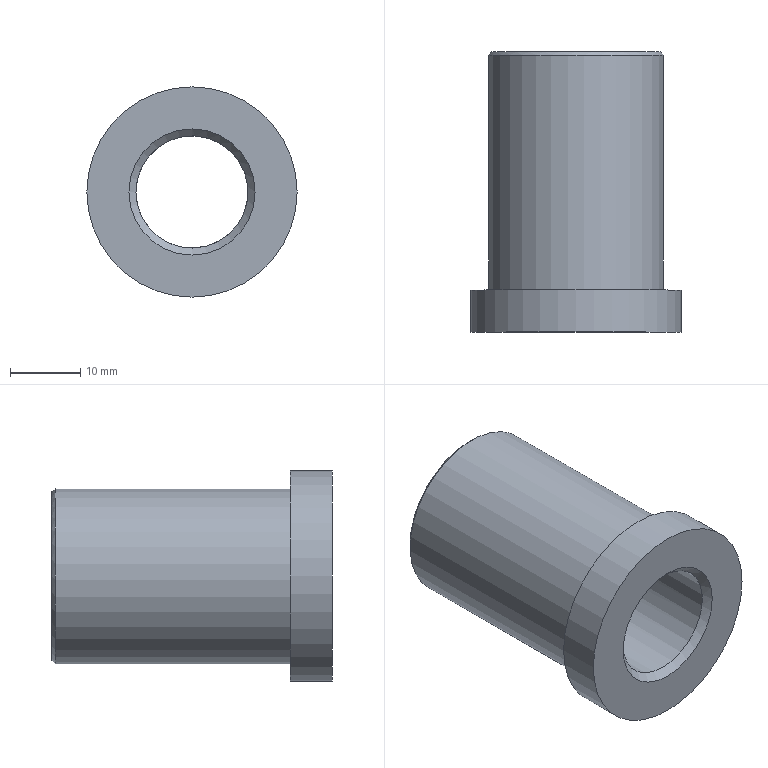Part | STEP file | GUIDE4_id94_x_t | 1 solid | 9 faces | box 30 x 40 x 30 mm | volume 12807 mm3 | cylinder 3 | plane 3 | cone 2 | other 1 | commonest cylinder face diameters 16 x1 25 x1 30 x1
STEP:
#1=CARTESIAN_POINT('',(115.,-109.5,43.));
#2=VERTEX_POINT('',#1);
#3=CARTESIAN_POINT('',(115.,-109.5,35.));
#4=DIRECTION('',(0.,-1.,0.));
#5=DIRECTION('',(0.,0.,1.));
#6=AXIS2_PLACEMENT_3D('',#3,#4,#5);
#7=CIRCLE('',#6,8.);
#8=EDGE_CURVE('',#2,#2,#7,.T.);
#9=ORIENTED_EDGE('',*,*,#8,.T.);
#10=EDGE_LOOP('',(#9));
#11=FACE_BOUND('',#10,.T.);
#12=CARTESIAN_POINT('',(115.433,-72.5,42.988));
#13=VERTEX_POINT('',#12);
#14=CARTESIAN_POINT('',(115.,-72.5,35.));
#15=DIRECTION('',(0.,-1.,0.));
#16=DIRECTION('',(0.05406,0.,0.9985));
#17=AXIS2_PLACEMENT_3D('',#14,#15,#16);
#18=CIRCLE('',#17,8.);
#19=EDGE_CURVE('',#13,#13,#18,.T.);
#20=ORIENTED_EDGE('',*,*,#19,.F.);
#21=EDGE_LOOP('',(#20));
#22=FACE_BOUND('',#21,.T.);
#23=CARTESIAN_POINT('',(115.,-70.5,35.));
#24=DIRECTION('',(0.,-1.,0.));
#25=DIRECTION('',(0.,0.,-1.));
#26=AXIS2_PLACEMENT_3D('',#23,#24,#25);
#27=CYLINDRICAL_SURFACE('',#26,8.);
#28=ADVANCED_FACE('',(#11,#22),#27,.F.);
#29=ORIENTED_EDGE('',*,*,#8,.F.);
#30=EDGE_LOOP('',(#29));
#31=FACE_BOUND('',#30,.T.);
#32=CARTESIAN_POINT('',(115.,-110.5,26.));
#33=VERTEX_POINT('',#32);
#34=CARTESIAN_POINT('',(115.,-110.5,35.));
#35=DIRECTION('',(0.,1.,0.));
#36=DIRECTION('',(0.,0.,-1.));
#37=AXIS2_PLACEMENT_3D('',#34,#35,#36);
#38=CIRCLE('',#37,9.);
#39=EDGE_CURVE('',#33,#33,#38,.T.);
#40=ORIENTED_EDGE('',*,*,#39,.F.);
#41=EDGE_LOOP('',(#40));
#42=FACE_BOUND('',#41,.T.);
#43=CARTESIAN_POINT('',(115.,-110.5,35.));
#44=DIRECTION('',(0.,-1.,0.));
#45=DIRECTION('',(0.,0.,-1.));
#46=AXIS2_PLACEMENT_3D('',#43,#44,#45);
#47=CONICAL_SURFACE('',#46,9.,45.);
#48=ADVANCED_FACE('',(#31,#42),#47,.F.);
#49=ORIENTED_EDGE('',*,*,#19,.T.);
#50=EDGE_LOOP('',(#49));
#51=FACE_BOUND('',#50,.T.);
#52=CARTESIAN_POINT('',(115.,-70.5,25.));
#53=VERTEX_POINT('',#52);
#54=CARTESIAN_POINT('',(115.,-70.5,45.));
#55=VERTEX_POINT('',#54);
#56=CARTESIAN_POINT('',(115.,-70.5,25.));
#57=CARTESIAN_POINT('',(95.,-70.5,25.));
#58=CARTESIAN_POINT('',(95.,-70.5,45.));
#59=CARTESIAN_POINT('',(115.,-70.5,45.));
#60=(BOUNDED_CURVE()B_SPLINE_CURVE(3,(#56,#57,#58,#59),.UNSPECIFIED.,.F.,.F.)B_SPLINE_CURVE_WITH_KNOTS((4,4),(0.,1.),.UNSPECIFIED.)CURVE()GEOMETRIC_REPRESENTATION_ITEM()RATIONAL_B_SPLINE_CURVE((1.,0.3333,0.3333,1.))REPRESENTATION_ITEM(''));
#61=EDGE_CURVE('',#53,#55,#60,.T.);
#62=ORIENTED_EDGE('',*,*,#61,.T.);
#63=CARTESIAN_POINT('',(115.,-70.5,45.));
#64=CARTESIAN_POINT('',(135.,-70.5,45.));
#65=CARTESIAN_POINT('',(135.,-70.5,25.));
#66=CARTESIAN_POINT('',(115.,-70.5,25.));
#67=(BOUNDED_CURVE()B_SPLINE_CURVE(3,(#63,#64,#65,#66),.UNSPECIFIED.,.F.,.F.)B_SPLINE_CURVE_WITH_KNOTS((4,4),(0.,1.),.UNSPECIFIED.)CURVE()GEOMETRIC_REPRESENTATION_ITEM()RATIONAL_B_SPLINE_CURVE((1.,0.3333,0.3333,1.))REPRESENTATION_ITEM(''));
#68=EDGE_CURVE('',#55,#53,#67,.T.);
#69=ORIENTED_EDGE('',*,*,#68,.T.);
#70=EDGE_LOOP('',(#62,#69));
#71=FACE_BOUND('',#70,.T.);
#72=CARTESIAN_POINT('',(115.541,-72.5,44.985));
#73=DIRECTION('',(-0.9985,0.,0.05406));
#74=DIRECTION('',(0.05406,0.,0.9985));
#75=AXIS2_PLACEMENT_3D('',#72,#73,#74);
#76=CIRCLE('',#75,2.);
#77=CARTESIAN_POINT('',(115.,-72.5,35.));
#78=DIRECTION('',(0.,-1.,0.));
#79=AXIS1_PLACEMENT('',#77,#78);
#80=SURFACE_OF_REVOLUTION('',#76,#79);
#81=ADVANCED_FACE('',(#51,#71),#80,.F.);
#82=ORIENTED_EDGE('',*,*,#39,.T.);
#83=EDGE_LOOP('',(#82));
#84=FACE_BOUND('',#83,.T.);
#85=CARTESIAN_POINT('',(115.,-110.5,50.));
#86=VERTEX_POINT('',#85);
#87=CARTESIAN_POINT('',(115.,-110.5,35.));
#88=DIRECTION('',(0.,1.,0.));
#89=DIRECTION('',(0.,0.,1.));
#90=AXIS2_PLACEMENT_3D('',#87,#88,#89);
#91=CIRCLE('',#90,15.);
#92=EDGE_CURVE('',#86,#86,#91,.T.);
#93=ORIENTED_EDGE('',*,*,#92,.F.);
#94=EDGE_LOOP('',(#93));
#95=FACE_BOUND('',#94,.T.);
#96=CARTESIAN_POINT('',(-200.,-110.5,-275.));
#97=DIRECTION('',(0.,-1.,0.));
#98=DIRECTION('',(0.,0.,-1.));
#99=AXIS2_PLACEMENT_3D('',#96,#97,#98);
#100=PLANE('',#99);
#101=ADVANCED_FACE('',(#84,#95),#100,.T.);
#102=ORIENTED_EDGE('',*,*,#68,.F.);
#103=ORIENTED_EDGE('',*,*,#61,.F.);
#104=EDGE_LOOP('',(#102,#103));
#105=FACE_BOUND('',#104,.T.);
#106=CARTESIAN_POINT('',(115.,-70.5,23.));
#107=VERTEX_POINT('',#106);
#108=CARTESIAN_POINT('',(115.,-70.5,35.));
#109=DIRECTION('',(0.,-1.,0.));
#110=DIRECTION('',(0.,0.,-1.));
#111=AXIS2_PLACEMENT_3D('',#108,#109,#110);
#112=CIRCLE('',#111,12.);
#113=EDGE_CURVE('',#107,#107,#112,.T.);
#114=ORIENTED_EDGE('',*,*,#113,.F.);
#115=EDGE_LOOP('',(#114));
#116=FACE_BOUND('',#115,.T.);
#117=CARTESIAN_POINT('',(-106.875,-70.5,-240.));
#118=DIRECTION('',(0.,-1.,0.));
#119=DIRECTION('',(0.,0.,-1.));
#120=AXIS2_PLACEMENT_3D('',#117,#118,#119);
#121=PLANE('',#120);
#122=ADVANCED_FACE('',(#105,#116),#121,.F.);
#123=CARTESIAN_POINT('',(115.,-104.5,50.));
#124=VERTEX_POINT('',#123);
#125=CARTESIAN_POINT('',(115.,-104.5,35.));
#126=DIRECTION('',(0.,1.,0.));
#127=DIRECTION('',(0.,0.,1.));
#128=AXIS2_PLACEMENT_3D('',#125,#126,#127);
#129=CIRCLE('',#128,15.);
#130=EDGE_CURVE('',#124,#124,#129,.T.);
#131=ORIENTED_EDGE('',*,*,#130,.F.);
#132=EDGE_LOOP('',(#131));
#133=FACE_BOUND('',#132,.T.);
#134=ORIENTED_EDGE('',*,*,#92,.T.);
#135=EDGE_LOOP('',(#134));
#136=FACE_BOUND('',#135,.T.);
#137=CARTESIAN_POINT('',(115.,-110.5,35.));
#138=DIRECTION('',(0.,1.,0.));
#139=DIRECTION('',(0.,0.,1.));
#140=AXIS2_PLACEMENT_3D('',#137,#138,#139);
#141=CYLINDRICAL_SURFACE('',#140,15.);
#142=ADVANCED_FACE('',(#133,#136),#141,.T.);
#143=CARTESIAN_POINT('',(115.,-71.,22.5));
#144=VERTEX_POINT('',#143);
#145=CARTESIAN_POINT('',(115.,-71.,35.));
#146=DIRECTION('',(0.,-1.,0.));
#147=DIRECTION('',(0.,0.,-1.));
#148=AXIS2_PLACEMENT_3D('',#145,#146,#147);
#149=CIRCLE('',#148,12.5);
#150=EDGE_CURVE('',#144,#144,#149,.T.);
#151=ORIENTED_EDGE('',*,*,#150,.F.);
#152=EDGE_LOOP('',(#151));
#153=FACE_BOUND('',#152,.T.);
#154=ORIENTED_EDGE('',*,*,#113,.T.);
#155=EDGE_LOOP('',(#154));
#156=FACE_BOUND('',#155,.T.);
#157=CARTESIAN_POINT('',(115.,-71.,35.));
#158=DIRECTION('',(0.,-1.,0.));
#159=DIRECTION('',(0.,0.,-1.));
#160=AXIS2_PLACEMENT_3D('',#157,#158,#159);
#161=CONICAL_SURFACE('',#160,12.5,45.);
#162=ADVANCED_FACE('',(#153,#156),#161,.T.);
#163=CARTESIAN_POINT('',(115.,-104.5,22.5));
#164=VERTEX_POINT('',#163);
#165=CARTESIAN_POINT('',(115.,-104.5,35.));
#166=DIRECTION('',(0.,1.,0.));
#167=DIRECTION('',(0.,0.,-1.));
#168=AXIS2_PLACEMENT_3D('',#165,#166,#167);
#169=CIRCLE('',#168,12.5);
#170=EDGE_CURVE('',#164,#164,#169,.T.);
#171=ORIENTED_EDGE('',*,*,#170,.F.);
#172=EDGE_LOOP('',(#171));
#173=FACE_BOUND('',#172,.T.);
#174=ORIENTED_EDGE('',*,*,#130,.T.);
#175=EDGE_LOOP('',(#174));
#176=FACE_BOUND('',#175,.T.);
#177=CARTESIAN_POINT('',(-200.,-104.5,275.));
#178=DIRECTION('',(0.,1.,0.));
#179=DIRECTION('',(0.,0.,1.));
#180=AXIS2_PLACEMENT_3D('',#177,#178,#179);
#181=PLANE('',#180);
#182=ADVANCED_FACE('',(#173,#176),#181,.T.);
#183=ORIENTED_EDGE('',*,*,#150,.T.);
#184=EDGE_LOOP('',(#183));
#185=FACE_BOUND('',#184,.T.);
#186=ORIENTED_EDGE('',*,*,#170,.T.);
#187=EDGE_LOOP('',(#186));
#188=FACE_BOUND('',#187,.T.);
#189=CARTESIAN_POINT('',(115.,-70.5,35.));
#190=DIRECTION('',(0.,-1.,0.));
#191=DIRECTION('',(0.,0.,-1.));
#192=AXIS2_PLACEMENT_3D('',#189,#190,#191);
#193=CYLINDRICAL_SURFACE('',#192,12.5);
#194=ADVANCED_FACE('',(#185,#188),#193,.T.);
#195=CLOSED_SHELL('',(#28,#48,#81,#101,#122,#142,#162,#182,#194));
#196=MANIFOLD_SOLID_BREP('',#195);
#197=(LENGTH_UNIT()NAMED_UNIT(*)SI_UNIT(.MILLI.,.METRE.));
#198=UNCERTAINTY_MEASURE_WITH_UNIT(LENGTH_MEASURE(0.0508),#197,'','');
#199=(NAMED_UNIT(*)PLANE_ANGLE_UNIT()SI_UNIT($,.RADIAN.));
#200=PLANE_ANGLE_MEASURE_WITH_UNIT(PLANE_ANGLE_MEASURE(0.01745),#199);
#201=DIMENSIONAL_EXPONENTS(0.,0.,0.,0.,0.,0.,0.);
#202=(CONVERSION_BASED_UNIT('DEGREE',#200)NAMED_UNIT(#201)PLANE_ANGLE_UNIT());
#203=(NAMED_UNIT(*)SI_UNIT($,.STERADIAN.)SOLID_ANGLE_UNIT());
#204=(GEOMETRIC_REPRESENTATION_CONTEXT(3)GLOBAL_UNCERTAINTY_ASSIGNED_CONTEXT((#198))GLOBAL_UNIT_ASSIGNED_CONTEXT((#197,#202,#203))REPRESENTATION_CONTEXT('',''));
#205=ADVANCED_BREP_SHAPE_REPRESENTATION('',(#196),#204);